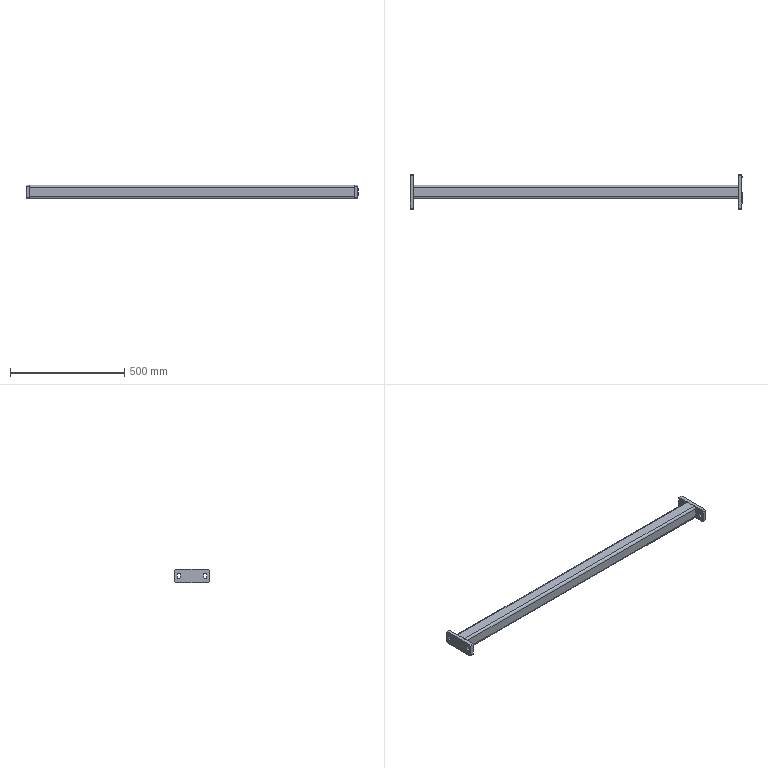Part | SolidWorks | features HoleWzd 2, ICE 1, MirrorSolid 1, WeldMemberFeat 1, WeldmentFeature 1 | 3 solids | 66 faces | box 1451 x 150 x 60 mm | volume 1723034 mm3 | plane 38 | cylinder 28 | commonest cylinder face diameters 13.5 x12 5 x8 10 x4 20 x4